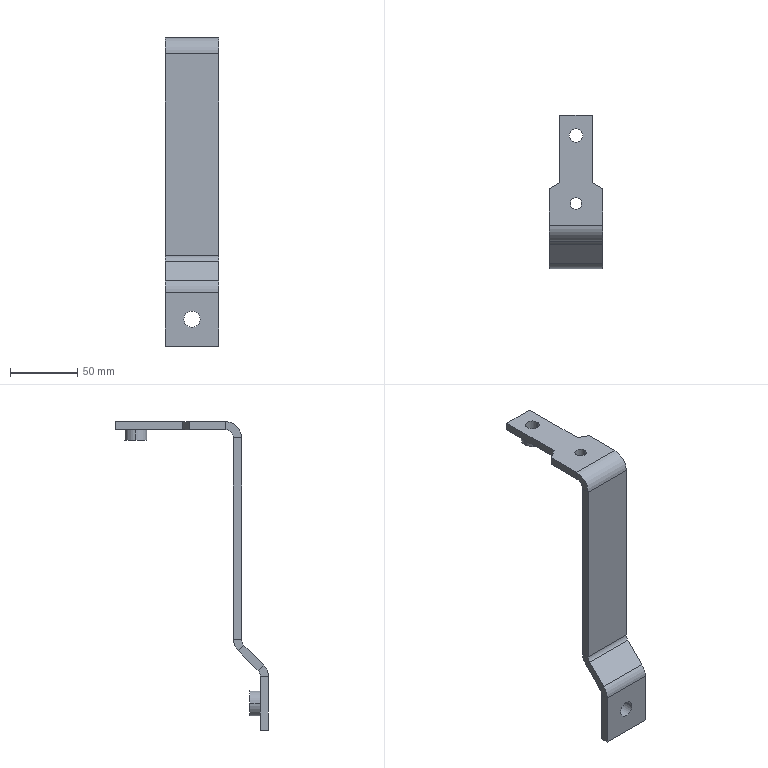Part | STEP file | 64586874 | 1 solid | 46 faces | box 40 x 113.5 x 229 mm | volume 72622 mm3 | plane 30 | cylinder 16 | commonest cylinder face diameters 12 x5 24 x3 8.5 x2 10 x2 16.5 x2 18.5 x2